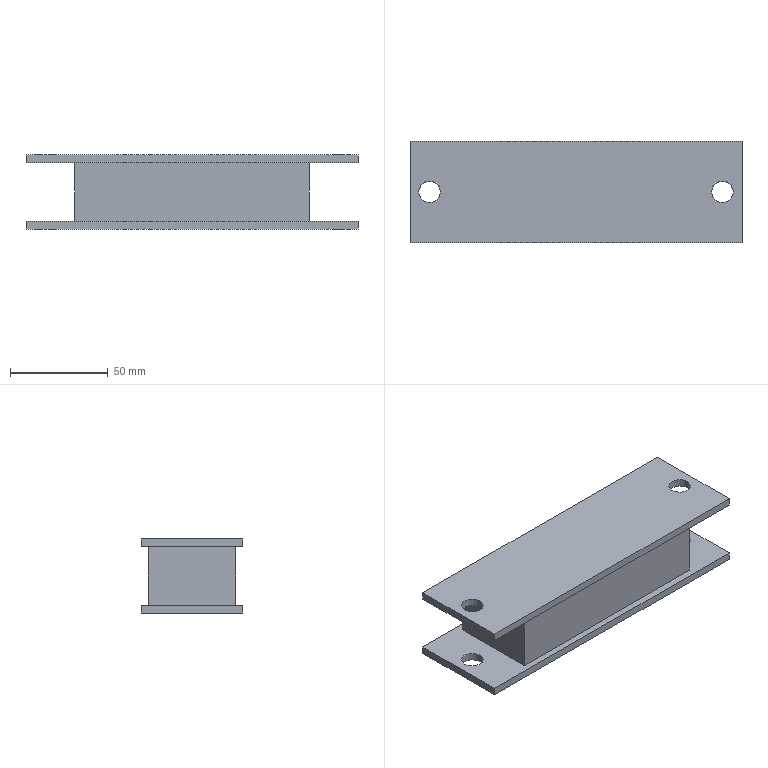Part | SolidWorks | features ICE 2, Extrusion 1, MirrorPattern 1, RefAxis 1 | 1 solid | 24 faces | box 170 x 52 x 38 mm | volume 231199 mm3 | plane 16 | cylinder 8 | commonest cylinder face diameters 11 x8
STEP:
#1=CARTESIAN_POINT('',(-80.5,0.,15.));
#2=VERTEX_POINT('',#1);
#3=CARTESIAN_POINT('',(-69.5,0.,15.));
#4=VERTEX_POINT('',#3);
#5=CARTESIAN_POINT('',(-75.,0.,15.));
#6=DIRECTION('',(0.,0.,1.));
#7=DIRECTION('',(1.,0.,0.));
#8=AXIS2_PLACEMENT_3D('',#5,#6,#7);
#9=CIRCLE('',#8,5.5);
#10=EDGE_CURVE('',#2,#4,#9,.T.);
#11=ORIENTED_EDGE('',*,*,#10,.F.);
#12=CARTESIAN_POINT('',(-80.5,0.,19.));
#13=VERTEX_POINT('',#12);
#14=CARTESIAN_POINT('',(-80.5,0.,-19.));
#15=DIRECTION('',(0.,0.,1.));
#16=VECTOR('',#15,1000.);
#17=LINE('',#14,#16);
#18=EDGE_CURVE('',#2,#13,#17,.T.);
#19=ORIENTED_EDGE('',*,*,#18,.T.);
#20=CARTESIAN_POINT('',(-69.5,0.,19.));
#21=VERTEX_POINT('',#20);
#22=CARTESIAN_POINT('',(-75.,0.,19.));
#23=DIRECTION('',(0.,0.,1.));
#24=DIRECTION('',(1.,0.,0.));
#25=AXIS2_PLACEMENT_3D('',#22,#23,#24);
#26=CIRCLE('',#25,5.5);
#27=EDGE_CURVE('',#13,#21,#26,.T.);
#28=ORIENTED_EDGE('',*,*,#27,.T.);
#29=CARTESIAN_POINT('',(-69.5,0.,-19.));
#30=DIRECTION('',(0.,0.,1.));
#31=VECTOR('',#30,1000.);
#32=LINE('',#29,#31);
#33=EDGE_CURVE('',#4,#21,#32,.T.);
#34=ORIENTED_EDGE('',*,*,#33,.F.);
#35=EDGE_LOOP('',(#11,#19,#28,#34));
#36=FACE_OUTER_BOUND('',#35,.T.);
#37=CARTESIAN_POINT('',(-75.,0.,-19.));
#38=DIRECTION('',(0.,0.,1.));
#39=DIRECTION('',(1.,0.,0.));
#40=AXIS2_PLACEMENT_3D('',#37,#38,#39);
#41=CYLINDRICAL_SURFACE('',#40,5.5);
#42=ADVANCED_FACE('',(#36),#41,.F.);
#43=CARTESIAN_POINT('',(69.5,0.,15.));
#44=VERTEX_POINT('',#43);
#45=CARTESIAN_POINT('',(80.5,0.,15.));
#46=VERTEX_POINT('',#45);
#47=CARTESIAN_POINT('',(75.,0.,15.));
#48=DIRECTION('',(0.,0.,1.));
#49=DIRECTION('',(1.,0.,0.));
#50=AXIS2_PLACEMENT_3D('',#47,#48,#49);
#51=CIRCLE('',#50,5.5);
#52=EDGE_CURVE('',#44,#46,#51,.T.);
#53=ORIENTED_EDGE('',*,*,#52,.F.);
#54=CARTESIAN_POINT('',(69.5,0.,19.));
#55=VERTEX_POINT('',#54);
#56=CARTESIAN_POINT('',(69.5,0.,-19.));
#57=DIRECTION('',(0.,0.,1.));
#58=VECTOR('',#57,1000.);
#59=LINE('',#56,#58);
#60=EDGE_CURVE('',#44,#55,#59,.T.);
#61=ORIENTED_EDGE('',*,*,#60,.T.);
#62=CARTESIAN_POINT('',(80.5,0.,19.));
#63=VERTEX_POINT('',#62);
#64=CARTESIAN_POINT('',(75.,0.,19.));
#65=DIRECTION('',(0.,0.,1.));
#66=DIRECTION('',(-1.,0.,0.));
#67=AXIS2_PLACEMENT_3D('',#64,#65,#66);
#68=CIRCLE('',#67,5.5);
#69=EDGE_CURVE('',#55,#63,#68,.T.);
#70=ORIENTED_EDGE('',*,*,#69,.T.);
#71=CARTESIAN_POINT('',(80.5,0.,-19.));
#72=DIRECTION('',(0.,0.,1.));
#73=VECTOR('',#72,1000.);
#74=LINE('',#71,#73);
#75=EDGE_CURVE('',#46,#63,#74,.T.);
#76=ORIENTED_EDGE('',*,*,#75,.F.);
#77=EDGE_LOOP('',(#53,#61,#70,#76));
#78=FACE_OUTER_BOUND('',#77,.T.);
#79=CARTESIAN_POINT('',(75.,0.,-19.));
#80=DIRECTION('',(0.,0.,1.));
#81=DIRECTION('',(1.,0.,0.));
#82=AXIS2_PLACEMENT_3D('',#79,#80,#81);
#83=CYLINDRICAL_SURFACE('',#82,5.5);
#84=ADVANCED_FACE('',(#78),#83,.F.);
#85=CARTESIAN_POINT('',(-80.5,0.,-19.));
#86=VERTEX_POINT('',#85);
#87=CARTESIAN_POINT('',(-69.5,0.,-19.));
#88=VERTEX_POINT('',#87);
#89=CARTESIAN_POINT('',(-75.,0.,-19.));
#90=DIRECTION('',(0.,0.,1.));
#91=DIRECTION('',(1.,0.,0.));
#92=AXIS2_PLACEMENT_3D('',#89,#90,#91);
#93=CIRCLE('',#92,5.5);
#94=EDGE_CURVE('',#86,#88,#93,.T.);
#95=ORIENTED_EDGE('',*,*,#94,.F.);
#96=CARTESIAN_POINT('',(-80.5,0.,-15.));
#97=VERTEX_POINT('',#96);
#98=CARTESIAN_POINT('',(-80.5,0.,-19.));
#99=DIRECTION('',(0.,0.,1.));
#100=VECTOR('',#99,1000.);
#101=LINE('',#98,#100);
#102=EDGE_CURVE('',#86,#97,#101,.T.);
#103=ORIENTED_EDGE('',*,*,#102,.T.);
#104=CARTESIAN_POINT('',(-69.5,0.,-15.));
#105=VERTEX_POINT('',#104);
#106=CARTESIAN_POINT('',(-75.,0.,-15.));
#107=DIRECTION('',(0.,0.,-1.));
#108=DIRECTION('',(-1.,0.,0.));
#109=AXIS2_PLACEMENT_3D('',#106,#107,#108);
#110=CIRCLE('',#109,5.5);
#111=EDGE_CURVE('',#105,#97,#110,.T.);
#112=ORIENTED_EDGE('',*,*,#111,.F.);
#113=CARTESIAN_POINT('',(-69.5,0.,-19.));
#114=DIRECTION('',(0.,0.,1.));
#115=VECTOR('',#114,1000.);
#116=LINE('',#113,#115);
#117=EDGE_CURVE('',#88,#105,#116,.T.);
#118=ORIENTED_EDGE('',*,*,#117,.F.);
#119=EDGE_LOOP('',(#95,#103,#112,#118));
#120=FACE_OUTER_BOUND('',#119,.T.);
#121=CARTESIAN_POINT('',(-75.,0.,-19.));
#122=DIRECTION('',(0.,0.,1.));
#123=DIRECTION('',(1.,0.,0.));
#124=AXIS2_PLACEMENT_3D('',#121,#122,#123);
#125=CYLINDRICAL_SURFACE('',#124,5.5);
#126=ADVANCED_FACE('',(#120),#125,.F.);
#127=CARTESIAN_POINT('',(69.5,0.,-19.));
#128=VERTEX_POINT('',#127);
#129=CARTESIAN_POINT('',(80.5,0.,-19.));
#130=VERTEX_POINT('',#129);
#131=CARTESIAN_POINT('',(75.,0.,-19.));
#132=DIRECTION('',(0.,0.,1.));
#133=DIRECTION('',(-1.,0.,0.));
#134=AXIS2_PLACEMENT_3D('',#131,#132,#133);
#135=CIRCLE('',#134,5.5);
#136=EDGE_CURVE('',#128,#130,#135,.T.);
#137=ORIENTED_EDGE('',*,*,#136,.F.);
#138=CARTESIAN_POINT('',(69.5,0.,-15.));
#139=VERTEX_POINT('',#138);
#140=CARTESIAN_POINT('',(69.5,0.,-19.));
#141=DIRECTION('',(0.,0.,1.));
#142=VECTOR('',#141,1000.);
#143=LINE('',#140,#142);
#144=EDGE_CURVE('',#128,#139,#143,.T.);
#145=ORIENTED_EDGE('',*,*,#144,.T.);
#146=CARTESIAN_POINT('',(80.5,0.,-15.));
#147=VERTEX_POINT('',#146);
#148=CARTESIAN_POINT('',(75.,0.,-15.));
#149=DIRECTION('',(0.,0.,-1.));
#150=DIRECTION('',(-1.,0.,0.));
#151=AXIS2_PLACEMENT_3D('',#148,#149,#150);
#152=CIRCLE('',#151,5.5);
#153=EDGE_CURVE('',#147,#139,#152,.T.);
#154=ORIENTED_EDGE('',*,*,#153,.F.);
#155=CARTESIAN_POINT('',(80.5,0.,-19.));
#156=DIRECTION('',(0.,0.,1.));
#157=VECTOR('',#156,1000.);
#158=LINE('',#155,#157);
#159=EDGE_CURVE('',#130,#147,#158,.T.);
#160=ORIENTED_EDGE('',*,*,#159,.F.);
#161=EDGE_LOOP('',(#137,#145,#154,#160));
#162=FACE_OUTER_BOUND('',#161,.T.);
#163=CARTESIAN_POINT('',(75.,0.,-19.));
#164=DIRECTION('',(0.,0.,1.));
#165=DIRECTION('',(1.,0.,0.));
#166=AXIS2_PLACEMENT_3D('',#163,#164,#165);
#167=CYLINDRICAL_SURFACE('',#166,5.5);
#168=ADVANCED_FACE('',(#162),#167,.F.);
#169=CARTESIAN_POINT('',(60.,-22.5,-15.));
#170=VERTEX_POINT('',#169);
#171=CARTESIAN_POINT('',(60.,22.5,-15.));
#172=VERTEX_POINT('',#171);
#173=CARTESIAN_POINT('',(60.,22.5,-15.));
#174=DIRECTION('',(0.,1.,0.));
#175=VECTOR('',#174,1000.);
#176=LINE('',#173,#175);
#177=EDGE_CURVE('',#170,#172,#176,.T.);
#178=ORIENTED_EDGE('',*,*,#177,.T.);
#179=CARTESIAN_POINT('',(60.,22.5,15.));
#180=VERTEX_POINT('',#179);
#181=CARTESIAN_POINT('',(60.,22.5,15.));
#182=DIRECTION('',(0.,0.,-1.));
#183=VECTOR('',#182,1000.);
#184=LINE('',#181,#183);
#185=EDGE_CURVE('',#180,#172,#184,.T.);
#186=ORIENTED_EDGE('',*,*,#185,.F.);
#187=CARTESIAN_POINT('',(60.,-22.5,15.));
#188=VERTEX_POINT('',#187);
#189=CARTESIAN_POINT('',(60.,22.5,15.));
#190=DIRECTION('',(0.,1.,0.));
#191=VECTOR('',#190,1000.);
#192=LINE('',#189,#191);
#193=EDGE_CURVE('',#188,#180,#192,.T.);
#194=ORIENTED_EDGE('',*,*,#193,.F.);
#195=CARTESIAN_POINT('',(60.,-22.5,15.));
#196=DIRECTION('',(0.,0.,-1.));
#197=VECTOR('',#196,1000.);
#198=LINE('',#195,#197);
#199=EDGE_CURVE('',#188,#170,#198,.T.);
#200=ORIENTED_EDGE('',*,*,#199,.T.);
#201=EDGE_LOOP('',(#178,#186,#194,#200));
#202=FACE_OUTER_BOUND('',#201,.T.);
#203=CARTESIAN_POINT('',(60.,22.5,15.));
#204=DIRECTION('',(-1.,0.,0.));
#205=DIRECTION('',(0.,0.,1.));
#206=AXIS2_PLACEMENT_3D('',#203,#204,#205);
#207=PLANE('',#206);
#208=ADVANCED_FACE('',(#202),#207,.F.);
#209=CARTESIAN_POINT('',(-60.,22.5,-15.));
#210=VERTEX_POINT('',#209);
#211=CARTESIAN_POINT('',(-60.,22.5,-15.));
#212=DIRECTION('',(-1.,0.,0.));
#213=VECTOR('',#212,1000.);
#214=LINE('',#211,#213);
#215=EDGE_CURVE('',#172,#210,#214,.T.);
#216=ORIENTED_EDGE('',*,*,#215,.T.);
#217=CARTESIAN_POINT('',(-60.,22.5,15.));
#218=VERTEX_POINT('',#217);
#219=CARTESIAN_POINT('',(-60.,22.5,15.));
#220=DIRECTION('',(0.,0.,-1.));
#221=VECTOR('',#220,1000.);
#222=LINE('',#219,#221);
#223=EDGE_CURVE('',#218,#210,#222,.T.);
#224=ORIENTED_EDGE('',*,*,#223,.F.);
#225=CARTESIAN_POINT('',(-60.,22.5,15.));
#226=DIRECTION('',(-1.,0.,0.));
#227=VECTOR('',#226,1000.);
#228=LINE('',#225,#227);
#229=EDGE_CURVE('',#180,#218,#228,.T.);
#230=ORIENTED_EDGE('',*,*,#229,.F.);
#231=ORIENTED_EDGE('',*,*,#185,.T.);
#232=EDGE_LOOP('',(#216,#224,#230,#231));
#233=FACE_OUTER_BOUND('',#232,.T.);
#234=CARTESIAN_POINT('',(-60.,22.5,15.));
#235=DIRECTION('',(0.,-1.,0.));
#236=DIRECTION('',(0.,0.,-1.));
#237=AXIS2_PLACEMENT_3D('',#234,#235,#236);
#238=PLANE('',#237);
#239=ADVANCED_FACE('',(#233),#238,.F.);
#240=CARTESIAN_POINT('',(-60.,-22.5,-15.));
#241=VERTEX_POINT('',#240);
#242=CARTESIAN_POINT('',(-60.,22.5,-15.));
#243=DIRECTION('',(0.,-1.,0.));
#244=VECTOR('',#243,1000.);
#245=LINE('',#242,#244);
#246=EDGE_CURVE('',#210,#241,#245,.T.);
#247=ORIENTED_EDGE('',*,*,#246,.T.);
#248=CARTESIAN_POINT('',(-60.,-22.5,15.));
#249=VERTEX_POINT('',#248);
#250=CARTESIAN_POINT('',(-60.,-22.5,15.));
#251=DIRECTION('',(0.,0.,-1.));
#252=VECTOR('',#251,1000.);
#253=LINE('',#250,#252);
#254=EDGE_CURVE('',#249,#241,#253,.T.);
#255=ORIENTED_EDGE('',*,*,#254,.F.);
#256=CARTESIAN_POINT('',(-60.,22.5,15.));
#257=DIRECTION('',(0.,-1.,0.));
#258=VECTOR('',#257,1000.);
#259=LINE('',#256,#258);
#260=EDGE_CURVE('',#218,#249,#259,.T.);
#261=ORIENTED_EDGE('',*,*,#260,.F.);
#262=ORIENTED_EDGE('',*,*,#223,.T.);
#263=EDGE_LOOP('',(#247,#255,#261,#262));
#264=FACE_OUTER_BOUND('',#263,.T.);
#265=CARTESIAN_POINT('',(-60.,22.5,15.));
#266=DIRECTION('',(1.,0.,0.));
#267=DIRECTION('',(0.,1.,0.));
#268=AXIS2_PLACEMENT_3D('',#265,#266,#267);
#269=PLANE('',#268);
#270=ADVANCED_FACE('',(#264),#269,.F.);
#271=CARTESIAN_POINT('',(-60.,-22.5,-15.));
#272=DIRECTION('',(1.,0.,0.));
#273=VECTOR('',#272,1000.);
#274=LINE('',#271,#273);
#275=EDGE_CURVE('',#241,#170,#274,.T.);
#276=ORIENTED_EDGE('',*,*,#275,.T.);
#277=ORIENTED_EDGE('',*,*,#199,.F.);
#278=CARTESIAN_POINT('',(-60.,-22.5,15.));
#279=DIRECTION('',(1.,0.,0.));
#280=VECTOR('',#279,1000.);
#281=LINE('',#278,#280);
#282=EDGE_CURVE('',#249,#188,#281,.T.);
#283=ORIENTED_EDGE('',*,*,#282,.F.);
#284=ORIENTED_EDGE('',*,*,#254,.T.);
#285=EDGE_LOOP('',(#276,#277,#283,#284));
#286=FACE_OUTER_BOUND('',#285,.T.);
#287=CARTESIAN_POINT('',(-60.,-22.5,15.));
#288=DIRECTION('',(0.,1.,0.));
#289=DIRECTION('',(0.,0.,1.));
#290=AXIS2_PLACEMENT_3D('',#287,#288,#289);
#291=PLANE('',#290);
#292=ADVANCED_FACE('',(#286),#291,.F.);
#293=CARTESIAN_POINT('',(-75.,0.,15.));
#294=DIRECTION('',(0.,0.,1.));
#295=DIRECTION('',(1.,0.,0.));
#296=AXIS2_PLACEMENT_3D('',#293,#294,#295);
#297=CIRCLE('',#296,5.5);
#298=EDGE_CURVE('',#4,#2,#297,.T.);
#299=ORIENTED_EDGE('',*,*,#298,.T.);
#300=ORIENTED_EDGE('',*,*,#10,.T.);
#301=EDGE_LOOP('',(#299,#300));
#302=FACE_BOUND('',#301,.T.);
#303=CARTESIAN_POINT('',(75.,0.,15.));
#304=DIRECTION('',(0.,0.,1.));
#305=DIRECTION('',(1.,0.,0.));
#306=AXIS2_PLACEMENT_3D('',#303,#304,#305);
#307=CIRCLE('',#306,5.5);
#308=EDGE_CURVE('',#46,#44,#307,.T.);
#309=ORIENTED_EDGE('',*,*,#308,.T.);
#310=ORIENTED_EDGE('',*,*,#52,.T.);
#311=EDGE_LOOP('',(#309,#310));
#312=FACE_BOUND('',#311,.T.);
#313=CARTESIAN_POINT('',(85.,-26.,15.));
#314=VERTEX_POINT('',#313);
#315=CARTESIAN_POINT('',(85.,26.,15.));
#316=VERTEX_POINT('',#315);
#317=CARTESIAN_POINT('',(85.,26.,15.));
#318=DIRECTION('',(0.,1.,0.));
#319=VECTOR('',#318,1000.);
#320=LINE('',#317,#319);
#321=EDGE_CURVE('',#314,#316,#320,.T.);
#322=ORIENTED_EDGE('',*,*,#321,.F.);
#323=CARTESIAN_POINT('',(-85.,-26.,15.));
#324=VERTEX_POINT('',#323);
#325=CARTESIAN_POINT('',(-85.,-26.,15.));
#326=DIRECTION('',(1.,0.,0.));
#327=VECTOR('',#326,1000.);
#328=LINE('',#325,#327);
#329=EDGE_CURVE('',#324,#314,#328,.T.);
#330=ORIENTED_EDGE('',*,*,#329,.F.);
#331=CARTESIAN_POINT('',(-85.,26.,15.));
#332=VERTEX_POINT('',#331);
#333=CARTESIAN_POINT('',(-85.,26.,15.));
#334=DIRECTION('',(0.,-1.,0.));
#335=VECTOR('',#334,1000.);
#336=LINE('',#333,#335);
#337=EDGE_CURVE('',#332,#324,#336,.T.);
#338=ORIENTED_EDGE('',*,*,#337,.F.);
#339=CARTESIAN_POINT('',(-85.,26.,15.));
#340=DIRECTION('',(-1.,0.,0.));
#341=VECTOR('',#340,1000.);
#342=LINE('',#339,#341);
#343=EDGE_CURVE('',#316,#332,#342,.T.);
#344=ORIENTED_EDGE('',*,*,#343,.F.);
#345=EDGE_LOOP('',(#322,#330,#338,#344));
#346=FACE_OUTER_BOUND('',#345,.T.);
#347=ORIENTED_EDGE('',*,*,#282,.T.);
#348=ORIENTED_EDGE('',*,*,#193,.T.);
#349=ORIENTED_EDGE('',*,*,#229,.T.);
#350=ORIENTED_EDGE('',*,*,#260,.T.);
#351=EDGE_LOOP('',(#347,#348,#349,#350));
#352=FACE_BOUND('',#351,.T.);
#353=CARTESIAN_POINT('',(0.,0.,15.));
#354=DIRECTION('',(0.,0.,1.));
#355=DIRECTION('',(1.,0.,0.));
#356=AXIS2_PLACEMENT_3D('',#353,#354,#355);
#357=PLANE('',#356);
#358=ADVANCED_FACE('',(#302,#312,#346,#352),#357,.F.);
#359=ORIENTED_EDGE('',*,*,#321,.T.);
#360=CARTESIAN_POINT('',(85.,26.,19.));
#361=VERTEX_POINT('',#360);
#362=CARTESIAN_POINT('',(85.,26.,19.));
#363=DIRECTION('',(0.,0.,-1.));
#364=VECTOR('',#363,1000.);
#365=LINE('',#362,#364);
#366=EDGE_CURVE('',#361,#316,#365,.T.);
#367=ORIENTED_EDGE('',*,*,#366,.F.);
#368=CARTESIAN_POINT('',(85.,-26.,19.));
#369=VERTEX_POINT('',#368);
#370=CARTESIAN_POINT('',(85.,26.,19.));
#371=DIRECTION('',(0.,1.,0.));
#372=VECTOR('',#371,1000.);
#373=LINE('',#370,#372);
#374=EDGE_CURVE('',#369,#361,#373,.T.);
#375=ORIENTED_EDGE('',*,*,#374,.F.);
#376=CARTESIAN_POINT('',(85.,-26.,19.));
#377=DIRECTION('',(0.,0.,-1.));
#378=VECTOR('',#377,1000.);
#379=LINE('',#376,#378);
#380=EDGE_CURVE('',#369,#314,#379,.T.);
#381=ORIENTED_EDGE('',*,*,#380,.T.);
#382=EDGE_LOOP('',(#359,#367,#375,#381));
#383=FACE_OUTER_BOUND('',#382,.T.);
#384=CARTESIAN_POINT('',(85.,26.,19.));
#385=DIRECTION('',(-1.,0.,0.));
#386=DIRECTION('',(0.,0.,1.));
#387=AXIS2_PLACEMENT_3D('',#384,#385,#386);
#388=PLANE('',#387);
#389=ADVANCED_FACE('',(#383),#388,.F.);
#390=ORIENTED_EDGE('',*,*,#343,.T.);
#391=CARTESIAN_POINT('',(-85.,26.,19.));
#392=VERTEX_POINT('',#391);
#393=CARTESIAN_POINT('',(-85.,26.,19.));
#394=DIRECTION('',(0.,0.,-1.));
#395=VECTOR('',#394,1000.);
#396=LINE('',#393,#395);
#397=EDGE_CURVE('',#392,#332,#396,.T.);
#398=ORIENTED_EDGE('',*,*,#397,.F.);
#399=CARTESIAN_POINT('',(-85.,26.,19.));
#400=DIRECTION('',(-1.,0.,0.));
#401=VECTOR('',#400,1000.);
#402=LINE('',#399,#401);
#403=EDGE_CURVE('',#361,#392,#402,.T.);
#404=ORIENTED_EDGE('',*,*,#403,.F.);
#405=ORIENTED_EDGE('',*,*,#366,.T.);
#406=EDGE_LOOP('',(#390,#398,#404,#405));
#407=FACE_OUTER_BOUND('',#406,.T.);
#408=CARTESIAN_POINT('',(-85.,26.,19.));
#409=DIRECTION('',(0.,-1.,0.));
#410=DIRECTION('',(0.,0.,-1.));
#411=AXIS2_PLACEMENT_3D('',#408,#409,#410);
#412=PLANE('',#411);
#413=ADVANCED_FACE('',(#407),#412,.F.);
#414=ORIENTED_EDGE('',*,*,#337,.T.);
#415=CARTESIAN_POINT('',(-85.,-26.,19.));
#416=VERTEX_POINT('',#415);
#417=CARTESIAN_POINT('',(-85.,-26.,19.));
#418=DIRECTION('',(0.,0.,-1.));
#419=VECTOR('',#418,1000.);
#420=LINE('',#417,#419);
#421=EDGE_CURVE('',#416,#324,#420,.T.);
#422=ORIENTED_EDGE('',*,*,#421,.F.);
#423=CARTESIAN_POINT('',(-85.,26.,19.));
#424=DIRECTION('',(0.,-1.,0.));
#425=VECTOR('',#424,1000.);
#426=LINE('',#423,#425);
#427=EDGE_CURVE('',#392,#416,#426,.T.);
#428=ORIENTED_EDGE('',*,*,#427,.F.);
#429=ORIENTED_EDGE('',*,*,#397,.T.);
#430=EDGE_LOOP('',(#414,#422,#428,#429));
#431=FACE_OUTER_BOUND('',#430,.T.);
#432=CARTESIAN_POINT('',(-85.,26.,19.));
#433=DIRECTION('',(1.,0.,0.));
#434=DIRECTION('',(0.,0.,-1.));
#435=AXIS2_PLACEMENT_3D('',#432,#433,#434);
#436=PLANE('',#435);
#437=ADVANCED_FACE('',(#431),#436,.F.);
#438=ORIENTED_EDGE('',*,*,#329,.T.);
#439=ORIENTED_EDGE('',*,*,#380,.F.);
#440=CARTESIAN_POINT('',(-85.,-26.,19.));
#441=DIRECTION('',(1.,0.,0.));
#442=VECTOR('',#441,1000.);
#443=LINE('',#440,#442);
#444=EDGE_CURVE('',#416,#369,#443,.T.);
#445=ORIENTED_EDGE('',*,*,#444,.F.);
#446=ORIENTED_EDGE('',*,*,#421,.T.);
#447=EDGE_LOOP('',(#438,#439,#445,#446));
#448=FACE_OUTER_BOUND('',#447,.T.);
#449=CARTESIAN_POINT('',(-85.,-26.,19.));
#450=DIRECTION('',(0.,1.,0.));
#451=DIRECTION('',(0.,0.,1.));
#452=AXIS2_PLACEMENT_3D('',#449,#450,#451);
#453=PLANE('',#452);
#454=ADVANCED_FACE('',(#448),#453,.F.);
#455=CARTESIAN_POINT('',(-75.,0.,19.));
#456=DIRECTION('',(0.,0.,1.));
#457=DIRECTION('',(1.,0.,0.));
#458=AXIS2_PLACEMENT_3D('',#455,#456,#457);
#459=CIRCLE('',#458,5.5);
#460=EDGE_CURVE('',#21,#13,#459,.T.);
#461=ORIENTED_EDGE('',*,*,#460,.F.);
#462=ORIENTED_EDGE('',*,*,#27,.F.);
#463=EDGE_LOOP('',(#461,#462));
#464=FACE_BOUND('',#463,.T.);
#465=CARTESIAN_POINT('',(75.,0.,19.));
#466=DIRECTION('',(0.,0.,1.));
#467=DIRECTION('',(-1.,0.,0.));
#468=AXIS2_PLACEMENT_3D('',#465,#466,#467);
#469=CIRCLE('',#468,5.5);
#470=EDGE_CURVE('',#63,#55,#469,.T.);
#471=ORIENTED_EDGE('',*,*,#470,.F.);
#472=ORIENTED_EDGE('',*,*,#69,.F.);
#473=EDGE_LOOP('',(#471,#472));
#474=FACE_BOUND('',#473,.T.);
#475=ORIENTED_EDGE('',*,*,#374,.T.);
#476=ORIENTED_EDGE('',*,*,#403,.T.);
#477=ORIENTED_EDGE('',*,*,#427,.T.);
#478=ORIENTED_EDGE('',*,*,#444,.T.);
#479=EDGE_LOOP('',(#475,#476,#477,#478));
#480=FACE_OUTER_BOUND('',#479,.T.);
#481=CARTESIAN_POINT('',(0.,0.,19.));
#482=DIRECTION('',(0.,0.,1.));
#483=DIRECTION('',(1.,0.,0.));
#484=AXIS2_PLACEMENT_3D('',#481,#482,#483);
#485=PLANE('',#484);
#486=ADVANCED_FACE('',(#464,#474,#480),#485,.T.);
#487=CARTESIAN_POINT('',(85.,-26.,-15.));
#488=VERTEX_POINT('',#487);
#489=CARTESIAN_POINT('',(85.,26.,-15.));
#490=VERTEX_POINT('',#489);
#491=CARTESIAN_POINT('',(85.,26.,-15.));
#492=DIRECTION('',(0.,1.,0.));
#493=VECTOR('',#492,1000.);
#494=LINE('',#491,#493);
#495=EDGE_CURVE('',#488,#490,#494,.T.);
#496=ORIENTED_EDGE('',*,*,#495,.F.);
#497=CARTESIAN_POINT('',(85.,-26.,-19.));
#498=VERTEX_POINT('',#497);
#499=CARTESIAN_POINT('',(85.,-26.,-19.));
#500=DIRECTION('',(0.,0.,1.));
#501=VECTOR('',#500,1000.);
#502=LINE('',#499,#501);
#503=EDGE_CURVE('',#498,#488,#502,.T.);
#504=ORIENTED_EDGE('',*,*,#503,.F.);
#505=CARTESIAN_POINT('',(85.,26.,-19.));
#506=VERTEX_POINT('',#505);
#507=CARTESIAN_POINT('',(85.,26.,-19.));
#508=DIRECTION('',(0.,1.,0.));
#509=VECTOR('',#508,1000.);
#510=LINE('',#507,#509);
#511=EDGE_CURVE('',#498,#506,#510,.T.);
#512=ORIENTED_EDGE('',*,*,#511,.T.);
#513=CARTESIAN_POINT('',(85.,26.,-19.));
#514=DIRECTION('',(0.,0.,1.));
#515=VECTOR('',#514,1000.);
#516=LINE('',#513,#515);
#517=EDGE_CURVE('',#506,#490,#516,.T.);
#518=ORIENTED_EDGE('',*,*,#517,.T.);
#519=EDGE_LOOP('',(#496,#504,#512,#518));
#520=FACE_OUTER_BOUND('',#519,.T.);
#521=CARTESIAN_POINT('',(85.,26.,-19.));
#522=DIRECTION('',(1.,0.,0.));
#523=DIRECTION('',(0.,0.,-1.));
#524=AXIS2_PLACEMENT_3D('',#521,#522,#523);
#525=PLANE('',#524);
#526=ADVANCED_FACE('',(#520),#525,.T.);
#527=CARTESIAN_POINT('',(-85.,-26.,-15.));
#528=VERTEX_POINT('',#527);
#529=CARTESIAN_POINT('',(-85.,-26.,-15.));
#530=DIRECTION('',(1.,0.,0.));
#531=VECTOR('',#530,1000.);
#532=LINE('',#529,#531);
#533=EDGE_CURVE('',#528,#488,#532,.T.);
#534=ORIENTED_EDGE('',*,*,#533,.F.);
#535=CARTESIAN_POINT('',(-85.,-26.,-19.));
#536=VERTEX_POINT('',#535);
#537=CARTESIAN_POINT('',(-85.,-26.,-19.));
#538=DIRECTION('',(0.,0.,1.));
#539=VECTOR('',#538,1000.);
#540=LINE('',#537,#539);
#541=EDGE_CURVE('',#536,#528,#540,.T.);
#542=ORIENTED_EDGE('',*,*,#541,.F.);
#543=CARTESIAN_POINT('',(-85.,-26.,-19.));
#544=DIRECTION('',(1.,0.,0.));
#545=VECTOR('',#544,1000.);
#546=LINE('',#543,#545);
#547=EDGE_CURVE('',#536,#498,#546,.T.);
#548=ORIENTED_EDGE('',*,*,#547,.T.);
#549=ORIENTED_EDGE('',*,*,#503,.T.);
#550=EDGE_LOOP('',(#534,#542,#548,#549));
#551=FACE_OUTER_BOUND('',#550,.T.);
#552=CARTESIAN_POINT('',(-85.,-26.,-19.));
#553=DIRECTION('',(0.,-1.,0.));
#554=DIRECTION('',(0.,0.,-1.));
#555=AXIS2_PLACEMENT_3D('',#552,#553,#554);
#556=PLANE('',#555);
#557=ADVANCED_FACE('',(#551),#556,.T.);
#558=CARTESIAN_POINT('',(-85.,26.,-15.));
#559=VERTEX_POINT('',#558);
#560=CARTESIAN_POINT('',(-85.,26.,-15.));
#561=DIRECTION('',(0.,-1.,0.));
#562=VECTOR('',#561,1000.);
#563=LINE('',#560,#562);
#564=EDGE_CURVE('',#559,#528,#563,.T.);
#565=ORIENTED_EDGE('',*,*,#564,.F.);
#566=CARTESIAN_POINT('',(-85.,26.,-19.));
#567=VERTEX_POINT('',#566);
#568=CARTESIAN_POINT('',(-85.,26.,-19.));
#569=DIRECTION('',(0.,0.,1.));
#570=VECTOR('',#569,1000.);
#571=LINE('',#568,#570);
#572=EDGE_CURVE('',#567,#559,#571,.T.);
#573=ORIENTED_EDGE('',*,*,#572,.F.);
#574=CARTESIAN_POINT('',(-85.,26.,-19.));
#575=DIRECTION('',(0.,-1.,0.));
#576=VECTOR('',#575,1000.);
#577=LINE('',#574,#576);
#578=EDGE_CURVE('',#567,#536,#577,.T.);
#579=ORIENTED_EDGE('',*,*,#578,.T.);
#580=ORIENTED_EDGE('',*,*,#541,.T.);
#581=EDGE_LOOP('',(#565,#573,#579,#580));
#582=FACE_OUTER_BOUND('',#581,.T.);
#583=CARTESIAN_POINT('',(-85.,26.,-19.));
#584=DIRECTION('',(-1.,0.,0.));
#585=DIRECTION('',(0.,0.,1.));
#586=AXIS2_PLACEMENT_3D('',#583,#584,#585);
#587=PLANE('',#586);
#588=ADVANCED_FACE('',(#582),#587,.T.);
#589=CARTESIAN_POINT('',(-85.,26.,-15.));
#590=DIRECTION('',(-1.,0.,0.));
#591=VECTOR('',#590,1000.);
#592=LINE('',#589,#591);
#593=EDGE_CURVE('',#490,#559,#592,.T.);
#594=ORIENTED_EDGE('',*,*,#593,.F.);
#595=ORIENTED_EDGE('',*,*,#517,.F.);
#596=CARTESIAN_POINT('',(-85.,26.,-19.));
#597=DIRECTION('',(-1.,0.,0.));
#598=VECTOR('',#597,1000.);
#599=LINE('',#596,#598);
#600=EDGE_CURVE('',#506,#567,#599,.T.);
#601=ORIENTED_EDGE('',*,*,#600,.T.);
#602=ORIENTED_EDGE('',*,*,#572,.T.);
#603=EDGE_LOOP('',(#594,#595,#601,#602));
#604=FACE_OUTER_BOUND('',#603,.T.);
#605=CARTESIAN_POINT('',(-85.,26.,-19.));
#606=DIRECTION('',(0.,1.,0.));
#607=DIRECTION('',(0.,0.,1.));
#608=AXIS2_PLACEMENT_3D('',#605,#606,#607);
#609=PLANE('',#608);
#610=ADVANCED_FACE('',(#604),#609,.T.);
#611=CARTESIAN_POINT('',(-75.,0.,-19.));
#612=DIRECTION('',(0.,0.,1.));
#613=DIRECTION('',(1.,0.,0.));
#614=AXIS2_PLACEMENT_3D('',#611,#612,#613);
#615=CIRCLE('',#614,5.5);
#616=EDGE_CURVE('',#88,#86,#615,.T.);
#617=ORIENTED_EDGE('',*,*,#616,.T.);
#618=ORIENTED_EDGE('',*,*,#94,.T.);
#619=EDGE_LOOP('',(#617,#618));
#620=FACE_BOUND('',#619,.T.);
#621=CARTESIAN_POINT('',(75.,0.,-19.));
#622=DIRECTION('',(0.,0.,1.));
#623=DIRECTION('',(-1.,0.,0.));
#624=AXIS2_PLACEMENT_3D('',#621,#622,#623);
#625=CIRCLE('',#624,5.5);
#626=EDGE_CURVE('',#130,#128,#625,.T.);
#627=ORIENTED_EDGE('',*,*,#626,.T.);
#628=ORIENTED_EDGE('',*,*,#136,.T.);
#629=EDGE_LOOP('',(#627,#628));
#630=FACE_BOUND('',#629,.T.);
#631=ORIENTED_EDGE('',*,*,#511,.F.);
#632=ORIENTED_EDGE('',*,*,#547,.F.);
#633=ORIENTED_EDGE('',*,*,#578,.F.);
#634=ORIENTED_EDGE('',*,*,#600,.F.);
#635=EDGE_LOOP('',(#631,#632,#633,#634));
#636=FACE_OUTER_BOUND('',#635,.T.);
#637=CARTESIAN_POINT('',(0.,0.,-19.));
#638=DIRECTION('',(0.,0.,-1.));
#639=DIRECTION('',(1.,0.,0.));
#640=AXIS2_PLACEMENT_3D('',#637,#638,#639);
#641=PLANE('',#640);
#642=ADVANCED_FACE('',(#620,#630,#636),#641,.T.);
#643=ORIENTED_EDGE('',*,*,#111,.T.);
#644=CARTESIAN_POINT('',(-75.,0.,-15.));
#645=DIRECTION('',(0.,0.,-1.));
#646=DIRECTION('',(-1.,0.,0.));
#647=AXIS2_PLACEMENT_3D('',#644,#645,#646);
#648=CIRCLE('',#647,5.5);
#649=EDGE_CURVE('',#97,#105,#648,.T.);
#650=ORIENTED_EDGE('',*,*,#649,.T.);
#651=EDGE_LOOP('',(#643,#650));
#652=FACE_BOUND('',#651,.T.);
#653=ORIENTED_EDGE('',*,*,#153,.T.);
#654=CARTESIAN_POINT('',(75.,0.,-15.));
#655=DIRECTION('',(0.,0.,-1.));
#656=DIRECTION('',(-1.,0.,0.));
#657=AXIS2_PLACEMENT_3D('',#654,#655,#656);
#658=CIRCLE('',#657,5.5);
#659=EDGE_CURVE('',#139,#147,#658,.T.);
#660=ORIENTED_EDGE('',*,*,#659,.T.);
#661=EDGE_LOOP('',(#653,#660));
#662=FACE_BOUND('',#661,.T.);
#663=ORIENTED_EDGE('',*,*,#177,.F.);
#664=ORIENTED_EDGE('',*,*,#275,.F.);
#665=ORIENTED_EDGE('',*,*,#246,.F.);
#666=ORIENTED_EDGE('',*,*,#215,.F.);
#667=EDGE_LOOP('',(#663,#664,#665,#666));
#668=FACE_BOUND('',#667,.T.);
#669=ORIENTED_EDGE('',*,*,#495,.T.);
#670=ORIENTED_EDGE('',*,*,#593,.T.);
#671=ORIENTED_EDGE('',*,*,#564,.T.);
#672=ORIENTED_EDGE('',*,*,#533,.T.);
#673=EDGE_LOOP('',(#669,#670,#671,#672));
#674=FACE_OUTER_BOUND('',#673,.T.);
#675=CARTESIAN_POINT('',(0.,0.,-15.));
#676=DIRECTION('',(0.,0.,-1.));
#677=DIRECTION('',(1.,0.,0.));
#678=AXIS2_PLACEMENT_3D('',#675,#676,#677);
#679=PLANE('',#678);
#680=ADVANCED_FACE('',(#652,#662,#668,#674),#679,.F.);
#681=ORIENTED_EDGE('',*,*,#144,.F.);
#682=ORIENTED_EDGE('',*,*,#626,.F.);
#683=ORIENTED_EDGE('',*,*,#159,.T.);
#684=ORIENTED_EDGE('',*,*,#659,.F.);
#685=EDGE_LOOP('',(#681,#682,#683,#684));
#686=FACE_OUTER_BOUND('',#685,.T.);
#687=CARTESIAN_POINT('',(75.,0.,-19.));
#688=DIRECTION('',(0.,0.,1.));
#689=DIRECTION('',(1.,0.,0.));
#690=AXIS2_PLACEMENT_3D('',#687,#688,#689);
#691=CYLINDRICAL_SURFACE('',#690,5.5);
#692=ADVANCED_FACE('',(#686),#691,.F.);
#693=ORIENTED_EDGE('',*,*,#102,.F.);
#694=ORIENTED_EDGE('',*,*,#616,.F.);
#695=ORIENTED_EDGE('',*,*,#117,.T.);
#696=ORIENTED_EDGE('',*,*,#649,.F.);
#697=EDGE_LOOP('',(#693,#694,#695,#696));
#698=FACE_OUTER_BOUND('',#697,.T.);
#699=CARTESIAN_POINT('',(-75.,0.,-19.));
#700=DIRECTION('',(0.,0.,1.));
#701=DIRECTION('',(1.,0.,0.));
#702=AXIS2_PLACEMENT_3D('',#699,#700,#701);
#703=CYLINDRICAL_SURFACE('',#702,5.5);
#704=ADVANCED_FACE('',(#698),#703,.F.);
#705=ORIENTED_EDGE('',*,*,#60,.F.);
#706=ORIENTED_EDGE('',*,*,#308,.F.);
#707=ORIENTED_EDGE('',*,*,#75,.T.);
#708=ORIENTED_EDGE('',*,*,#470,.T.);
#709=EDGE_LOOP('',(#705,#706,#707,#708));
#710=FACE_OUTER_BOUND('',#709,.T.);
#711=CARTESIAN_POINT('',(75.,0.,-19.));
#712=DIRECTION('',(0.,0.,1.));
#713=DIRECTION('',(1.,0.,0.));
#714=AXIS2_PLACEMENT_3D('',#711,#712,#713);
#715=CYLINDRICAL_SURFACE('',#714,5.5);
#716=ADVANCED_FACE('',(#710),#715,.F.);
#717=ORIENTED_EDGE('',*,*,#18,.F.);
#718=ORIENTED_EDGE('',*,*,#298,.F.);
#719=ORIENTED_EDGE('',*,*,#33,.T.);
#720=ORIENTED_EDGE('',*,*,#460,.T.);
#721=EDGE_LOOP('',(#717,#718,#719,#720));
#722=FACE_OUTER_BOUND('',#721,.T.);
#723=CARTESIAN_POINT('',(-75.,0.,-19.));
#724=DIRECTION('',(0.,0.,1.));
#725=DIRECTION('',(1.,0.,0.));
#726=AXIS2_PLACEMENT_3D('',#723,#724,#725);
#727=CYLINDRICAL_SURFACE('',#726,5.5);
#728=ADVANCED_FACE('',(#722),#727,.F.);
#729=CLOSED_SHELL('',(#42,#84,#126,#168,#208,#239,#270,#292,#358,#389,#413,#437,#454,#486,#526,#557,#588,#610,#642,#680,#692,#704,#716,#728));
#730=MANIFOLD_SOLID_BREP('',#729);
#731=CARTESIAN_POINT('',(0.,0.,0.));
#732=DIRECTION('',(0.,0.,1.));
#733=DIRECTION('',(1.,0.,0.));
#734=AXIS2_PLACEMENT_3D('',#731,#732,#733);
#735=(LENGTH_UNIT()NAMED_UNIT(*)SI_UNIT(.MILLI.,.METRE.));
#736=UNCERTAINTY_MEASURE_WITH_UNIT(LENGTH_MEASURE(0.00001),#735,'','');
#737=(NAMED_UNIT(*)PLANE_ANGLE_UNIT()SI_UNIT($,.RADIAN.));
#738=(NAMED_UNIT(*)SI_UNIT($,.STERADIAN.)SOLID_ANGLE_UNIT());
#739=(GEOMETRIC_REPRESENTATION_CONTEXT(3)GLOBAL_UNCERTAINTY_ASSIGNED_CONTEXT((#736))GLOBAL_UNIT_ASSIGNED_CONTEXT((#735,#737,#738))REPRESENTATION_CONTEXT('',''));
#740=ADVANCED_BREP_SHAPE_REPRESENTATION('',(#730,#734),#739);